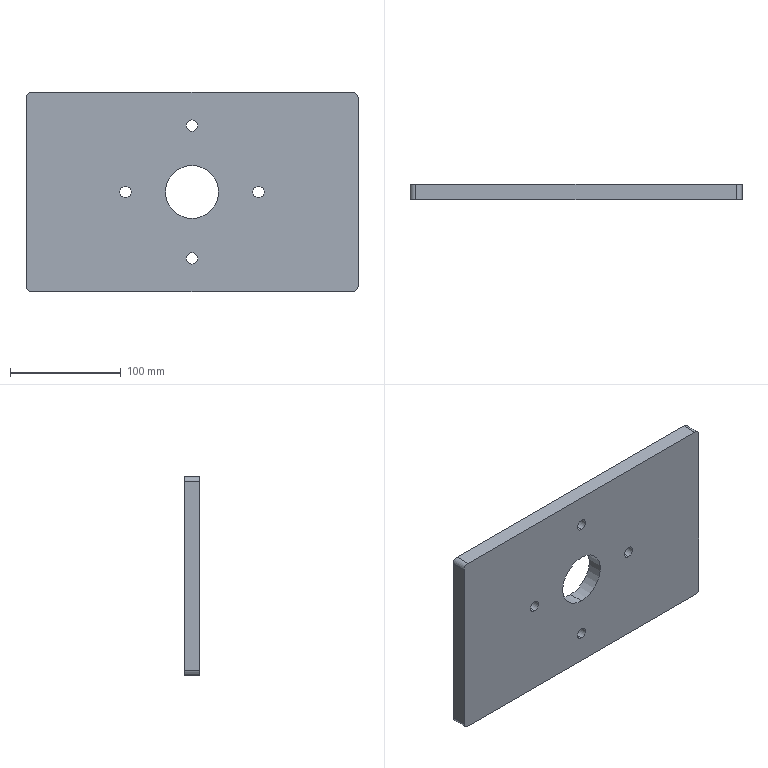Part | SolidWorks | features BaseBody 1 | 1 solid | 20 faces | box 300 x 14 x 180 mm | volume 725790 mm3 | cylinder 14 | plane 6 | commonest cylinder face diameters 10.2 x8 10 x4 48 x2
STEP:
#1=CARTESIAN_POINT('',(0.,0.,-24.));
#2=VERTEX_POINT('',#1);
#3=CARTESIAN_POINT('',(0.,0.,24.));
#4=VERTEX_POINT('',#3);
#5=CARTESIAN_POINT('',(0.,0.,0.));
#6=DIRECTION('',(0.,1.,0.));
#7=DIRECTION('',(0.,0.,1.));
#8=AXIS2_PLACEMENT_3D('',#5,#6,#7);
#9=CIRCLE('',#8,24.);
#10=EDGE_CURVE('',#2,#4,#9,.T.);
#11=ORIENTED_EDGE('',*,*,#10,.F.);
#12=CARTESIAN_POINT('',(0.,14.,-24.));
#13=VERTEX_POINT('',#12);
#14=CARTESIAN_POINT('',(0.,0.,-24.));
#15=DIRECTION('',(0.,1.,0.));
#16=VECTOR('',#15,1000.);
#17=LINE('',#14,#16);
#18=EDGE_CURVE('',#2,#13,#17,.T.);
#19=ORIENTED_EDGE('',*,*,#18,.T.);
#20=CARTESIAN_POINT('',(0.,14.,24.));
#21=VERTEX_POINT('',#20);
#22=CARTESIAN_POINT('',(0.,14.,0.));
#23=DIRECTION('',(0.,1.,0.));
#24=DIRECTION('',(0.,0.,1.));
#25=AXIS2_PLACEMENT_3D('',#22,#23,#24);
#26=CIRCLE('',#25,24.);
#27=EDGE_CURVE('',#13,#21,#26,.T.);
#28=ORIENTED_EDGE('',*,*,#27,.T.);
#29=CARTESIAN_POINT('',(0.,0.,24.));
#30=DIRECTION('',(0.,1.,0.));
#31=VECTOR('',#30,1000.);
#32=LINE('',#29,#31);
#33=EDGE_CURVE('',#4,#21,#32,.T.);
#34=ORIENTED_EDGE('',*,*,#33,.F.);
#35=EDGE_LOOP('',(#11,#19,#28,#34));
#36=FACE_OUTER_BOUND('',#35,.T.);
#37=CARTESIAN_POINT('',(0.,0.,0.));
#38=DIRECTION('',(0.,1.,0.));
#39=DIRECTION('',(0.,0.,1.));
#40=AXIS2_PLACEMENT_3D('',#37,#38,#39);
#41=CYLINDRICAL_SURFACE('',#40,24.);
#42=ADVANCED_FACE('',(#36),#41,.F.);
#43=CARTESIAN_POINT('',(0.,0.,-65.1));
#44=VERTEX_POINT('',#43);
#45=CARTESIAN_POINT('',(0.,0.,-54.9));
#46=VERTEX_POINT('',#45);
#47=CARTESIAN_POINT('',(0.,0.,-60.));
#48=DIRECTION('',(0.,1.,0.));
#49=DIRECTION('',(0.,0.,1.));
#50=AXIS2_PLACEMENT_3D('',#47,#48,#49);
#51=CIRCLE('',#50,5.1);
#52=EDGE_CURVE('',#44,#46,#51,.T.);
#53=ORIENTED_EDGE('',*,*,#52,.F.);
#54=CARTESIAN_POINT('',(0.,14.,-65.1));
#55=VERTEX_POINT('',#54);
#56=CARTESIAN_POINT('',(0.,14.,-65.1));
#57=DIRECTION('',(0.,1.,0.));
#58=VECTOR('',#57,1000.);
#59=LINE('',#56,#58);
#60=EDGE_CURVE('',#44,#55,#59,.T.);
#61=ORIENTED_EDGE('',*,*,#60,.T.);
#62=CARTESIAN_POINT('',(0.,14.,-54.9));
#63=VERTEX_POINT('',#62);
#64=CARTESIAN_POINT('',(0.,14.,-60.));
#65=DIRECTION('',(0.,1.,0.));
#66=DIRECTION('',(0.,0.,1.));
#67=AXIS2_PLACEMENT_3D('',#64,#65,#66);
#68=CIRCLE('',#67,5.1);
#69=EDGE_CURVE('',#55,#63,#68,.T.);
#70=ORIENTED_EDGE('',*,*,#69,.T.);
#71=CARTESIAN_POINT('',(0.,14.,-54.9));
#72=DIRECTION('',(0.,1.,0.));
#73=VECTOR('',#72,1000.);
#74=LINE('',#71,#73);
#75=EDGE_CURVE('',#46,#63,#74,.T.);
#76=ORIENTED_EDGE('',*,*,#75,.F.);
#77=EDGE_LOOP('',(#53,#61,#70,#76));
#78=FACE_OUTER_BOUND('',#77,.T.);
#79=CARTESIAN_POINT('',(0.,14.,-60.));
#80=DIRECTION('',(0.,1.,0.));
#81=DIRECTION('',(0.,0.,1.));
#82=AXIS2_PLACEMENT_3D('',#79,#80,#81);
#83=CYLINDRICAL_SURFACE('',#82,5.1);
#84=ADVANCED_FACE('',(#78),#83,.F.);
#85=CARTESIAN_POINT('',(-60.,0.,-5.1));
#86=VERTEX_POINT('',#85);
#87=CARTESIAN_POINT('',(-60.,0.,5.1));
#88=VERTEX_POINT('',#87);
#89=CARTESIAN_POINT('',(-60.,0.,0.));
#90=DIRECTION('',(0.,1.,0.));
#91=DIRECTION('',(0.,0.,1.));
#92=AXIS2_PLACEMENT_3D('',#89,#90,#91);
#93=CIRCLE('',#92,5.1);
#94=EDGE_CURVE('',#86,#88,#93,.T.);
#95=ORIENTED_EDGE('',*,*,#94,.F.);
#96=CARTESIAN_POINT('',(-60.,14.,-5.1));
#97=VERTEX_POINT('',#96);
#98=CARTESIAN_POINT('',(-60.,14.,-5.1));
#99=DIRECTION('',(0.,1.,0.));
#100=VECTOR('',#99,1000.);
#101=LINE('',#98,#100);
#102=EDGE_CURVE('',#86,#97,#101,.T.);
#103=ORIENTED_EDGE('',*,*,#102,.T.);
#104=CARTESIAN_POINT('',(-60.,14.,5.1));
#105=VERTEX_POINT('',#104);
#106=CARTESIAN_POINT('',(-60.,14.,0.));
#107=DIRECTION('',(0.,1.,0.));
#108=DIRECTION('',(0.,0.,1.));
#109=AXIS2_PLACEMENT_3D('',#106,#107,#108);
#110=CIRCLE('',#109,5.1);
#111=EDGE_CURVE('',#97,#105,#110,.T.);
#112=ORIENTED_EDGE('',*,*,#111,.T.);
#113=CARTESIAN_POINT('',(-60.,14.,5.1));
#114=DIRECTION('',(0.,1.,0.));
#115=VECTOR('',#114,1000.);
#116=LINE('',#113,#115);
#117=EDGE_CURVE('',#88,#105,#116,.T.);
#118=ORIENTED_EDGE('',*,*,#117,.F.);
#119=EDGE_LOOP('',(#95,#103,#112,#118));
#120=FACE_OUTER_BOUND('',#119,.T.);
#121=CARTESIAN_POINT('',(-60.,14.,0.));
#122=DIRECTION('',(0.,1.,0.));
#123=DIRECTION('',(0.,0.,1.));
#124=AXIS2_PLACEMENT_3D('',#121,#122,#123);
#125=CYLINDRICAL_SURFACE('',#124,5.1);
#126=ADVANCED_FACE('',(#120),#125,.F.);
#127=CARTESIAN_POINT('',(0.,0.,54.9));
#128=VERTEX_POINT('',#127);
#129=CARTESIAN_POINT('',(0.,0.,65.1));
#130=VERTEX_POINT('',#129);
#131=CARTESIAN_POINT('',(0.,0.,60.));
#132=DIRECTION('',(0.,1.,0.));
#133=DIRECTION('',(0.,0.,1.));
#134=AXIS2_PLACEMENT_3D('',#131,#132,#133);
#135=CIRCLE('',#134,5.1);
#136=EDGE_CURVE('',#128,#130,#135,.T.);
#137=ORIENTED_EDGE('',*,*,#136,.F.);
#138=CARTESIAN_POINT('',(0.,14.,54.9));
#139=VERTEX_POINT('',#138);
#140=CARTESIAN_POINT('',(0.,14.,54.9));
#141=DIRECTION('',(0.,1.,0.));
#142=VECTOR('',#141,1000.);
#143=LINE('',#140,#142);
#144=EDGE_CURVE('',#128,#139,#143,.T.);
#145=ORIENTED_EDGE('',*,*,#144,.T.);
#146=CARTESIAN_POINT('',(0.,14.,65.1));
#147=VERTEX_POINT('',#146);
#148=CARTESIAN_POINT('',(0.,14.,60.));
#149=DIRECTION('',(0.,1.,0.));
#150=DIRECTION('',(0.,0.,1.));
#151=AXIS2_PLACEMENT_3D('',#148,#149,#150);
#152=CIRCLE('',#151,5.1);
#153=EDGE_CURVE('',#139,#147,#152,.T.);
#154=ORIENTED_EDGE('',*,*,#153,.T.);
#155=CARTESIAN_POINT('',(0.,14.,65.1));
#156=DIRECTION('',(0.,1.,0.));
#157=VECTOR('',#156,1000.);
#158=LINE('',#155,#157);
#159=EDGE_CURVE('',#130,#147,#158,.T.);
#160=ORIENTED_EDGE('',*,*,#159,.F.);
#161=EDGE_LOOP('',(#137,#145,#154,#160));
#162=FACE_OUTER_BOUND('',#161,.T.);
#163=CARTESIAN_POINT('',(0.,14.,60.));
#164=DIRECTION('',(0.,1.,0.));
#165=DIRECTION('',(0.,0.,1.));
#166=AXIS2_PLACEMENT_3D('',#163,#164,#165);
#167=CYLINDRICAL_SURFACE('',#166,5.1);
#168=ADVANCED_FACE('',(#162),#167,.F.);
#169=CARTESIAN_POINT('',(60.,0.,-5.1));
#170=VERTEX_POINT('',#169);
#171=CARTESIAN_POINT('',(60.,0.,5.1));
#172=VERTEX_POINT('',#171);
#173=CARTESIAN_POINT('',(60.,0.,0.));
#174=DIRECTION('',(0.,1.,0.));
#175=DIRECTION('',(0.,0.,1.));
#176=AXIS2_PLACEMENT_3D('',#173,#174,#175);
#177=CIRCLE('',#176,5.1);
#178=EDGE_CURVE('',#170,#172,#177,.T.);
#179=ORIENTED_EDGE('',*,*,#178,.F.);
#180=CARTESIAN_POINT('',(60.,14.,-5.1));
#181=VERTEX_POINT('',#180);
#182=CARTESIAN_POINT('',(60.,14.,-5.1));
#183=DIRECTION('',(0.,1.,0.));
#184=VECTOR('',#183,1000.);
#185=LINE('',#182,#184);
#186=EDGE_CURVE('',#170,#181,#185,.T.);
#187=ORIENTED_EDGE('',*,*,#186,.T.);
#188=CARTESIAN_POINT('',(60.,14.,5.1));
#189=VERTEX_POINT('',#188);
#190=CARTESIAN_POINT('',(60.,14.,0.));
#191=DIRECTION('',(0.,1.,0.));
#192=DIRECTION('',(0.,0.,1.));
#193=AXIS2_PLACEMENT_3D('',#190,#191,#192);
#194=CIRCLE('',#193,5.1);
#195=EDGE_CURVE('',#181,#189,#194,.T.);
#196=ORIENTED_EDGE('',*,*,#195,.T.);
#197=CARTESIAN_POINT('',(60.,14.,5.1));
#198=DIRECTION('',(0.,1.,0.));
#199=VECTOR('',#198,1000.);
#200=LINE('',#197,#199);
#201=EDGE_CURVE('',#172,#189,#200,.T.);
#202=ORIENTED_EDGE('',*,*,#201,.F.);
#203=EDGE_LOOP('',(#179,#187,#196,#202));
#204=FACE_OUTER_BOUND('',#203,.T.);
#205=CARTESIAN_POINT('',(60.,14.,0.));
#206=DIRECTION('',(0.,1.,0.));
#207=DIRECTION('',(0.,0.,1.));
#208=AXIS2_PLACEMENT_3D('',#205,#206,#207);
#209=CYLINDRICAL_SURFACE('',#208,5.1);
#210=ADVANCED_FACE('',(#204),#209,.F.);
#211=CARTESIAN_POINT('',(145.,14.,-90.));
#212=VERTEX_POINT('',#211);
#213=CARTESIAN_POINT('',(150.,14.,-85.));
#214=VERTEX_POINT('',#213);
#215=CARTESIAN_POINT('',(145.,14.,-85.));
#216=DIRECTION('',(0.,-1.,0.));
#217=DIRECTION('',(0.,0.,-1.));
#218=AXIS2_PLACEMENT_3D('',#215,#216,#217);
#219=CIRCLE('',#218,5.);
#220=EDGE_CURVE('',#212,#214,#219,.T.);
#221=ORIENTED_EDGE('',*,*,#220,.F.);
#222=CARTESIAN_POINT('',(-145.,14.,-90.));
#223=VERTEX_POINT('',#222);
#224=CARTESIAN_POINT('',(0.,14.,-90.));
#225=DIRECTION('',(1.,0.,0.));
#226=VECTOR('',#225,1000.);
#227=LINE('',#224,#226);
#228=EDGE_CURVE('',#223,#212,#227,.T.);
#229=ORIENTED_EDGE('',*,*,#228,.F.);
#230=CARTESIAN_POINT('',(-150.,14.,-85.));
#231=VERTEX_POINT('',#230);
#232=CARTESIAN_POINT('',(-145.,14.,-85.));
#233=DIRECTION('',(0.,-1.,0.));
#234=DIRECTION('',(0.,0.,-1.));
#235=AXIS2_PLACEMENT_3D('',#232,#233,#234);
#236=CIRCLE('',#235,5.);
#237=EDGE_CURVE('',#231,#223,#236,.T.);
#238=ORIENTED_EDGE('',*,*,#237,.F.);
#239=CARTESIAN_POINT('',(-150.,14.,85.));
#240=VERTEX_POINT('',#239);
#241=CARTESIAN_POINT('',(-150.,14.,0.));
#242=DIRECTION('',(0.,0.,-1.));
#243=VECTOR('',#242,1000.);
#244=LINE('',#241,#243);
#245=EDGE_CURVE('',#240,#231,#244,.T.);
#246=ORIENTED_EDGE('',*,*,#245,.F.);
#247=CARTESIAN_POINT('',(-145.,14.,90.));
#248=VERTEX_POINT('',#247);
#249=CARTESIAN_POINT('',(-145.,14.,85.));
#250=DIRECTION('',(0.,-1.,0.));
#251=DIRECTION('',(0.,0.,-1.));
#252=AXIS2_PLACEMENT_3D('',#249,#250,#251);
#253=CIRCLE('',#252,5.);
#254=EDGE_CURVE('',#248,#240,#253,.T.);
#255=ORIENTED_EDGE('',*,*,#254,.F.);
#256=CARTESIAN_POINT('',(145.,14.,90.));
#257=VERTEX_POINT('',#256);
#258=CARTESIAN_POINT('',(0.,14.,90.));
#259=DIRECTION('',(-1.,0.,0.));
#260=VECTOR('',#259,1000.);
#261=LINE('',#258,#260);
#262=EDGE_CURVE('',#257,#248,#261,.T.);
#263=ORIENTED_EDGE('',*,*,#262,.F.);
#264=CARTESIAN_POINT('',(150.,14.,85.));
#265=VERTEX_POINT('',#264);
#266=CARTESIAN_POINT('',(145.,14.,85.));
#267=DIRECTION('',(0.,-1.,0.));
#268=DIRECTION('',(0.,0.,-1.));
#269=AXIS2_PLACEMENT_3D('',#266,#267,#268);
#270=CIRCLE('',#269,5.);
#271=EDGE_CURVE('',#265,#257,#270,.T.);
#272=ORIENTED_EDGE('',*,*,#271,.F.);
#273=CARTESIAN_POINT('',(150.,14.,0.));
#274=DIRECTION('',(0.,0.,1.));
#275=VECTOR('',#274,1000.);
#276=LINE('',#273,#275);
#277=EDGE_CURVE('',#214,#265,#276,.T.);
#278=ORIENTED_EDGE('',*,*,#277,.F.);
#279=EDGE_LOOP('',(#221,#229,#238,#246,#255,#263,#272,#278));
#280=FACE_OUTER_BOUND('',#279,.T.);
#281=CARTESIAN_POINT('',(0.,14.,0.));
#282=DIRECTION('',(0.,1.,0.));
#283=DIRECTION('',(0.,0.,1.));
#284=AXIS2_PLACEMENT_3D('',#281,#282,#283);
#285=CIRCLE('',#284,24.);
#286=EDGE_CURVE('',#21,#13,#285,.T.);
#287=ORIENTED_EDGE('',*,*,#286,.F.);
#288=ORIENTED_EDGE('',*,*,#27,.F.);
#289=EDGE_LOOP('',(#287,#288));
#290=FACE_BOUND('',#289,.T.);
#291=CARTESIAN_POINT('',(0.,14.,-60.));
#292=DIRECTION('',(0.,1.,0.));
#293=DIRECTION('',(0.,0.,1.));
#294=AXIS2_PLACEMENT_3D('',#291,#292,#293);
#295=CIRCLE('',#294,5.1);
#296=EDGE_CURVE('',#63,#55,#295,.T.);
#297=ORIENTED_EDGE('',*,*,#296,.F.);
#298=ORIENTED_EDGE('',*,*,#69,.F.);
#299=EDGE_LOOP('',(#297,#298));
#300=FACE_BOUND('',#299,.T.);
#301=CARTESIAN_POINT('',(-60.,14.,0.));
#302=DIRECTION('',(0.,1.,0.));
#303=DIRECTION('',(0.,0.,1.));
#304=AXIS2_PLACEMENT_3D('',#301,#302,#303);
#305=CIRCLE('',#304,5.1);
#306=EDGE_CURVE('',#105,#97,#305,.T.);
#307=ORIENTED_EDGE('',*,*,#306,.F.);
#308=ORIENTED_EDGE('',*,*,#111,.F.);
#309=EDGE_LOOP('',(#307,#308));
#310=FACE_BOUND('',#309,.T.);
#311=CARTESIAN_POINT('',(0.,14.,60.));
#312=DIRECTION('',(0.,1.,0.));
#313=DIRECTION('',(0.,0.,1.));
#314=AXIS2_PLACEMENT_3D('',#311,#312,#313);
#315=CIRCLE('',#314,5.1);
#316=EDGE_CURVE('',#147,#139,#315,.T.);
#317=ORIENTED_EDGE('',*,*,#316,.F.);
#318=ORIENTED_EDGE('',*,*,#153,.F.);
#319=EDGE_LOOP('',(#317,#318));
#320=FACE_BOUND('',#319,.T.);
#321=CARTESIAN_POINT('',(60.,14.,0.));
#322=DIRECTION('',(0.,1.,0.));
#323=DIRECTION('',(0.,0.,1.));
#324=AXIS2_PLACEMENT_3D('',#321,#322,#323);
#325=CIRCLE('',#324,5.1);
#326=EDGE_CURVE('',#189,#181,#325,.T.);
#327=ORIENTED_EDGE('',*,*,#326,.F.);
#328=ORIENTED_EDGE('',*,*,#195,.F.);
#329=EDGE_LOOP('',(#327,#328));
#330=FACE_BOUND('',#329,.T.);
#331=CARTESIAN_POINT('',(0.,14.,0.));
#332=DIRECTION('',(0.,-1.,0.));
#333=DIRECTION('',(0.,0.,-1.));
#334=AXIS2_PLACEMENT_3D('',#331,#332,#333);
#335=PLANE('',#334);
#336=ADVANCED_FACE('',(#280,#290,#300,#310,#320,#330),#335,.F.);
#337=CARTESIAN_POINT('',(150.,0.,-85.));
#338=VERTEX_POINT('',#337);
#339=CARTESIAN_POINT('',(150.,14.,-85.));
#340=DIRECTION('',(0.,-1.,0.));
#341=VECTOR('',#340,1000.);
#342=LINE('',#339,#341);
#343=EDGE_CURVE('',#214,#338,#342,.T.);
#344=ORIENTED_EDGE('',*,*,#343,.F.);
#345=ORIENTED_EDGE('',*,*,#277,.T.);
#346=CARTESIAN_POINT('',(150.,0.,85.));
#347=VERTEX_POINT('',#346);
#348=CARTESIAN_POINT('',(150.,14.,85.));
#349=DIRECTION('',(0.,1.,0.));
#350=VECTOR('',#349,1000.);
#351=LINE('',#348,#350);
#352=EDGE_CURVE('',#347,#265,#351,.T.);
#353=ORIENTED_EDGE('',*,*,#352,.F.);
#354=CARTESIAN_POINT('',(150.,0.,90.));
#355=DIRECTION('',(0.,0.,1.));
#356=VECTOR('',#355,1000.);
#357=LINE('',#354,#356);
#358=EDGE_CURVE('',#338,#347,#357,.T.);
#359=ORIENTED_EDGE('',*,*,#358,.F.);
#360=EDGE_LOOP('',(#344,#345,#353,#359));
#361=FACE_OUTER_BOUND('',#360,.T.);
#362=CARTESIAN_POINT('',(150.,14.,90.));
#363=DIRECTION('',(-1.,0.,0.));
#364=DIRECTION('',(0.,0.,1.));
#365=AXIS2_PLACEMENT_3D('',#362,#363,#364);
#366=PLANE('',#365);
#367=ADVANCED_FACE('',(#361),#366,.F.);
#368=CARTESIAN_POINT('',(145.,0.,-90.));
#369=VERTEX_POINT('',#368);
#370=CARTESIAN_POINT('',(145.,0.,-85.));
#371=DIRECTION('',(0.,1.,0.));
#372=DIRECTION('',(0.,0.,-1.));
#373=AXIS2_PLACEMENT_3D('',#370,#371,#372);
#374=CIRCLE('',#373,5.);
#375=EDGE_CURVE('',#338,#369,#374,.T.);
#376=ORIENTED_EDGE('',*,*,#375,.T.);
#377=CARTESIAN_POINT('',(145.,14.,-90.));
#378=DIRECTION('',(0.,1.,0.));
#379=VECTOR('',#378,1000.);
#380=LINE('',#377,#379);
#381=EDGE_CURVE('',#369,#212,#380,.T.);
#382=ORIENTED_EDGE('',*,*,#381,.T.);
#383=ORIENTED_EDGE('',*,*,#220,.T.);
#384=ORIENTED_EDGE('',*,*,#343,.T.);
#385=EDGE_LOOP('',(#376,#382,#383,#384));
#386=FACE_OUTER_BOUND('',#385,.T.);
#387=CARTESIAN_POINT('',(145.,14.,-85.));
#388=DIRECTION('',(0.,-1.,0.));
#389=DIRECTION('',(0.,0.,-1.));
#390=AXIS2_PLACEMENT_3D('',#387,#388,#389);
#391=CYLINDRICAL_SURFACE('',#390,5.);
#392=ADVANCED_FACE('',(#386),#391,.T.);
#393=ORIENTED_EDGE('',*,*,#381,.F.);
#394=CARTESIAN_POINT('',(-145.,0.,-90.));
#395=VERTEX_POINT('',#394);
#396=CARTESIAN_POINT('',(-150.,0.,-90.));
#397=DIRECTION('',(1.,0.,0.));
#398=VECTOR('',#397,1000.);
#399=LINE('',#396,#398);
#400=EDGE_CURVE('',#395,#369,#399,.T.);
#401=ORIENTED_EDGE('',*,*,#400,.F.);
#402=CARTESIAN_POINT('',(-145.,14.,-90.));
#403=DIRECTION('',(0.,-1.,0.));
#404=VECTOR('',#403,1000.);
#405=LINE('',#402,#404);
#406=EDGE_CURVE('',#223,#395,#405,.T.);
#407=ORIENTED_EDGE('',*,*,#406,.F.);
#408=ORIENTED_EDGE('',*,*,#228,.T.);
#409=EDGE_LOOP('',(#393,#401,#407,#408));
#410=FACE_OUTER_BOUND('',#409,.T.);
#411=CARTESIAN_POINT('',(-150.,14.,-90.));
#412=DIRECTION('',(0.,0.,1.));
#413=DIRECTION('',(1.,0.,0.));
#414=AXIS2_PLACEMENT_3D('',#411,#412,#413);
#415=PLANE('',#414);
#416=ADVANCED_FACE('',(#410),#415,.F.);
#417=CARTESIAN_POINT('',(-150.,0.,-85.));
#418=VERTEX_POINT('',#417);
#419=CARTESIAN_POINT('',(-145.,0.,-85.));
#420=DIRECTION('',(0.,1.,0.));
#421=DIRECTION('',(0.,0.,-1.));
#422=AXIS2_PLACEMENT_3D('',#419,#420,#421);
#423=CIRCLE('',#422,5.);
#424=EDGE_CURVE('',#395,#418,#423,.T.);
#425=ORIENTED_EDGE('',*,*,#424,.T.);
#426=CARTESIAN_POINT('',(-150.,14.,-85.));
#427=DIRECTION('',(0.,1.,0.));
#428=VECTOR('',#427,1000.);
#429=LINE('',#426,#428);
#430=EDGE_CURVE('',#418,#231,#429,.T.);
#431=ORIENTED_EDGE('',*,*,#430,.T.);
#432=ORIENTED_EDGE('',*,*,#237,.T.);
#433=ORIENTED_EDGE('',*,*,#406,.T.);
#434=EDGE_LOOP('',(#425,#431,#432,#433));
#435=FACE_OUTER_BOUND('',#434,.T.);
#436=CARTESIAN_POINT('',(-145.,14.,-85.));
#437=DIRECTION('',(0.,-1.,0.));
#438=DIRECTION('',(0.,0.,-1.));
#439=AXIS2_PLACEMENT_3D('',#436,#437,#438);
#440=CYLINDRICAL_SURFACE('',#439,5.);
#441=ADVANCED_FACE('',(#435),#440,.T.);
#442=CARTESIAN_POINT('',(-150.,0.,85.));
#443=VERTEX_POINT('',#442);
#444=CARTESIAN_POINT('',(-150.,14.,85.));
#445=DIRECTION('',(0.,-1.,0.));
#446=VECTOR('',#445,1000.);
#447=LINE('',#444,#446);
#448=EDGE_CURVE('',#240,#443,#447,.T.);
#449=ORIENTED_EDGE('',*,*,#448,.F.);
#450=ORIENTED_EDGE('',*,*,#245,.T.);
#451=ORIENTED_EDGE('',*,*,#430,.F.);
#452=CARTESIAN_POINT('',(-150.,0.,90.));
#453=DIRECTION('',(0.,0.,-1.));
#454=VECTOR('',#453,1000.);
#455=LINE('',#452,#454);
#456=EDGE_CURVE('',#443,#418,#455,.T.);
#457=ORIENTED_EDGE('',*,*,#456,.F.);
#458=EDGE_LOOP('',(#449,#450,#451,#457));
#459=FACE_OUTER_BOUND('',#458,.T.);
#460=CARTESIAN_POINT('',(-150.,14.,90.));
#461=DIRECTION('',(1.,0.,0.));
#462=DIRECTION('',(0.,0.,-1.));
#463=AXIS2_PLACEMENT_3D('',#460,#461,#462);
#464=PLANE('',#463);
#465=ADVANCED_FACE('',(#459),#464,.F.);
#466=CARTESIAN_POINT('',(-145.,0.,90.));
#467=VERTEX_POINT('',#466);
#468=CARTESIAN_POINT('',(-145.,0.,85.));
#469=DIRECTION('',(0.,1.,0.));
#470=DIRECTION('',(0.,0.,-1.));
#471=AXIS2_PLACEMENT_3D('',#468,#469,#470);
#472=CIRCLE('',#471,5.);
#473=EDGE_CURVE('',#443,#467,#472,.T.);
#474=ORIENTED_EDGE('',*,*,#473,.T.);
#475=CARTESIAN_POINT('',(-145.,14.,90.));
#476=DIRECTION('',(0.,1.,0.));
#477=VECTOR('',#476,1000.);
#478=LINE('',#475,#477);
#479=EDGE_CURVE('',#467,#248,#478,.T.);
#480=ORIENTED_EDGE('',*,*,#479,.T.);
#481=ORIENTED_EDGE('',*,*,#254,.T.);
#482=ORIENTED_EDGE('',*,*,#448,.T.);
#483=EDGE_LOOP('',(#474,#480,#481,#482));
#484=FACE_OUTER_BOUND('',#483,.T.);
#485=CARTESIAN_POINT('',(-145.,14.,85.));
#486=DIRECTION('',(0.,-1.,0.));
#487=DIRECTION('',(0.,0.,-1.));
#488=AXIS2_PLACEMENT_3D('',#485,#486,#487);
#489=CYLINDRICAL_SURFACE('',#488,5.);
#490=ADVANCED_FACE('',(#484),#489,.T.);
#491=CARTESIAN_POINT('',(145.,0.,90.));
#492=VERTEX_POINT('',#491);
#493=CARTESIAN_POINT('',(145.,14.,90.));
#494=DIRECTION('',(0.,-1.,0.));
#495=VECTOR('',#494,1000.);
#496=LINE('',#493,#495);
#497=EDGE_CURVE('',#257,#492,#496,.T.);
#498=ORIENTED_EDGE('',*,*,#497,.F.);
#499=ORIENTED_EDGE('',*,*,#262,.T.);
#500=ORIENTED_EDGE('',*,*,#479,.F.);
#501=CARTESIAN_POINT('',(-150.,0.,90.));
#502=DIRECTION('',(-1.,0.,0.));
#503=VECTOR('',#502,1000.);
#504=LINE('',#501,#503);
#505=EDGE_CURVE('',#492,#467,#504,.T.);
#506=ORIENTED_EDGE('',*,*,#505,.F.);
#507=EDGE_LOOP('',(#498,#499,#500,#506));
#508=FACE_OUTER_BOUND('',#507,.T.);
#509=CARTESIAN_POINT('',(-150.,14.,90.));
#510=DIRECTION('',(0.,0.,-1.));
#511=DIRECTION('',(-1.,0.,0.));
#512=AXIS2_PLACEMENT_3D('',#509,#510,#511);
#513=PLANE('',#512);
#514=ADVANCED_FACE('',(#508),#513,.F.);
#515=CARTESIAN_POINT('',(145.,0.,85.));
#516=DIRECTION('',(0.,1.,0.));
#517=DIRECTION('',(0.,0.,-1.));
#518=AXIS2_PLACEMENT_3D('',#515,#516,#517);
#519=CIRCLE('',#518,5.);
#520=EDGE_CURVE('',#492,#347,#519,.T.);
#521=ORIENTED_EDGE('',*,*,#520,.T.);
#522=ORIENTED_EDGE('',*,*,#352,.T.);
#523=ORIENTED_EDGE('',*,*,#271,.T.);
#524=ORIENTED_EDGE('',*,*,#497,.T.);
#525=EDGE_LOOP('',(#521,#522,#523,#524));
#526=FACE_OUTER_BOUND('',#525,.T.);
#527=CARTESIAN_POINT('',(145.,14.,85.));
#528=DIRECTION('',(0.,-1.,0.));
#529=DIRECTION('',(0.,0.,-1.));
#530=AXIS2_PLACEMENT_3D('',#527,#528,#529);
#531=CYLINDRICAL_SURFACE('',#530,5.);
#532=ADVANCED_FACE('',(#526),#531,.T.);
#533=ORIENTED_EDGE('',*,*,#18,.F.);
#534=CARTESIAN_POINT('',(0.,0.,0.));
#535=DIRECTION('',(0.,1.,0.));
#536=DIRECTION('',(0.,0.,1.));
#537=AXIS2_PLACEMENT_3D('',#534,#535,#536);
#538=CIRCLE('',#537,24.);
#539=EDGE_CURVE('',#4,#2,#538,.T.);
#540=ORIENTED_EDGE('',*,*,#539,.F.);
#541=ORIENTED_EDGE('',*,*,#33,.T.);
#542=ORIENTED_EDGE('',*,*,#286,.T.);
#543=EDGE_LOOP('',(#533,#540,#541,#542));
#544=FACE_OUTER_BOUND('',#543,.T.);
#545=CARTESIAN_POINT('',(0.,0.,0.));
#546=DIRECTION('',(0.,1.,0.));
#547=DIRECTION('',(0.,0.,1.));
#548=AXIS2_PLACEMENT_3D('',#545,#546,#547);
#549=CYLINDRICAL_SURFACE('',#548,24.);
#550=ADVANCED_FACE('',(#544),#549,.F.);
#551=ORIENTED_EDGE('',*,*,#60,.F.);
#552=CARTESIAN_POINT('',(0.,0.,-60.));
#553=DIRECTION('',(0.,1.,0.));
#554=DIRECTION('',(0.,0.,1.));
#555=AXIS2_PLACEMENT_3D('',#552,#553,#554);
#556=CIRCLE('',#555,5.1);
#557=EDGE_CURVE('',#46,#44,#556,.T.);
#558=ORIENTED_EDGE('',*,*,#557,.F.);
#559=ORIENTED_EDGE('',*,*,#75,.T.);
#560=ORIENTED_EDGE('',*,*,#296,.T.);
#561=EDGE_LOOP('',(#551,#558,#559,#560));
#562=FACE_OUTER_BOUND('',#561,.T.);
#563=CARTESIAN_POINT('',(0.,14.,-60.));
#564=DIRECTION('',(0.,1.,0.));
#565=DIRECTION('',(0.,0.,1.));
#566=AXIS2_PLACEMENT_3D('',#563,#564,#565);
#567=CYLINDRICAL_SURFACE('',#566,5.1);
#568=ADVANCED_FACE('',(#562),#567,.F.);
#569=ORIENTED_EDGE('',*,*,#102,.F.);
#570=CARTESIAN_POINT('',(-60.,0.,0.));
#571=DIRECTION('',(0.,1.,0.));
#572=DIRECTION('',(0.,0.,1.));
#573=AXIS2_PLACEMENT_3D('',#570,#571,#572);
#574=CIRCLE('',#573,5.1);
#575=EDGE_CURVE('',#88,#86,#574,.T.);
#576=ORIENTED_EDGE('',*,*,#575,.F.);
#577=ORIENTED_EDGE('',*,*,#117,.T.);
#578=ORIENTED_EDGE('',*,*,#306,.T.);
#579=EDGE_LOOP('',(#569,#576,#577,#578));
#580=FACE_OUTER_BOUND('',#579,.T.);
#581=CARTESIAN_POINT('',(-60.,14.,0.));
#582=DIRECTION('',(0.,1.,0.));
#583=DIRECTION('',(0.,0.,1.));
#584=AXIS2_PLACEMENT_3D('',#581,#582,#583);
#585=CYLINDRICAL_SURFACE('',#584,5.1);
#586=ADVANCED_FACE('',(#580),#585,.F.);
#587=ORIENTED_EDGE('',*,*,#144,.F.);
#588=CARTESIAN_POINT('',(0.,0.,60.));
#589=DIRECTION('',(0.,1.,0.));
#590=DIRECTION('',(0.,0.,1.));
#591=AXIS2_PLACEMENT_3D('',#588,#589,#590);
#592=CIRCLE('',#591,5.1);
#593=EDGE_CURVE('',#130,#128,#592,.T.);
#594=ORIENTED_EDGE('',*,*,#593,.F.);
#595=ORIENTED_EDGE('',*,*,#159,.T.);
#596=ORIENTED_EDGE('',*,*,#316,.T.);
#597=EDGE_LOOP('',(#587,#594,#595,#596));
#598=FACE_OUTER_BOUND('',#597,.T.);
#599=CARTESIAN_POINT('',(0.,14.,60.));
#600=DIRECTION('',(0.,1.,0.));
#601=DIRECTION('',(0.,0.,1.));
#602=AXIS2_PLACEMENT_3D('',#599,#600,#601);
#603=CYLINDRICAL_SURFACE('',#602,5.1);
#604=ADVANCED_FACE('',(#598),#603,.F.);
#605=ORIENTED_EDGE('',*,*,#186,.F.);
#606=CARTESIAN_POINT('',(60.,0.,0.));
#607=DIRECTION('',(0.,1.,0.));
#608=DIRECTION('',(0.,0.,1.));
#609=AXIS2_PLACEMENT_3D('',#606,#607,#608);
#610=CIRCLE('',#609,5.1);
#611=EDGE_CURVE('',#172,#170,#610,.T.);
#612=ORIENTED_EDGE('',*,*,#611,.F.);
#613=ORIENTED_EDGE('',*,*,#201,.T.);
#614=ORIENTED_EDGE('',*,*,#326,.T.);
#615=EDGE_LOOP('',(#605,#612,#613,#614));
#616=FACE_OUTER_BOUND('',#615,.T.);
#617=CARTESIAN_POINT('',(60.,14.,0.));
#618=DIRECTION('',(0.,1.,0.));
#619=DIRECTION('',(0.,0.,1.));
#620=AXIS2_PLACEMENT_3D('',#617,#618,#619);
#621=CYLINDRICAL_SURFACE('',#620,5.1);
#622=ADVANCED_FACE('',(#616),#621,.F.);
#623=ORIENTED_EDGE('',*,*,#456,.T.);
#624=ORIENTED_EDGE('',*,*,#424,.F.);
#625=ORIENTED_EDGE('',*,*,#400,.T.);
#626=ORIENTED_EDGE('',*,*,#375,.F.);
#627=ORIENTED_EDGE('',*,*,#358,.T.);
#628=ORIENTED_EDGE('',*,*,#520,.F.);
#629=ORIENTED_EDGE('',*,*,#505,.T.);
#630=ORIENTED_EDGE('',*,*,#473,.F.);
#631=EDGE_LOOP('',(#623,#624,#625,#626,#627,#628,#629,#630));
#632=FACE_OUTER_BOUND('',#631,.T.);
#633=ORIENTED_EDGE('',*,*,#539,.T.);
#634=ORIENTED_EDGE('',*,*,#10,.T.);
#635=EDGE_LOOP('',(#633,#634));
#636=FACE_BOUND('',#635,.T.);
#637=ORIENTED_EDGE('',*,*,#557,.T.);
#638=ORIENTED_EDGE('',*,*,#52,.T.);
#639=EDGE_LOOP('',(#637,#638));
#640=FACE_BOUND('',#639,.T.);
#641=ORIENTED_EDGE('',*,*,#575,.T.);
#642=ORIENTED_EDGE('',*,*,#94,.T.);
#643=EDGE_LOOP('',(#641,#642));
#644=FACE_BOUND('',#643,.T.);
#645=ORIENTED_EDGE('',*,*,#593,.T.);
#646=ORIENTED_EDGE('',*,*,#136,.T.);
#647=EDGE_LOOP('',(#645,#646));
#648=FACE_BOUND('',#647,.T.);
#649=ORIENTED_EDGE('',*,*,#611,.T.);
#650=ORIENTED_EDGE('',*,*,#178,.T.);
#651=EDGE_LOOP('',(#649,#650));
#652=FACE_BOUND('',#651,.T.);
#653=CARTESIAN_POINT('',(0.,0.,0.));
#654=DIRECTION('',(0.,-1.,0.));
#655=DIRECTION('',(0.,0.,-1.));
#656=AXIS2_PLACEMENT_3D('',#653,#654,#655);
#657=PLANE('',#656);
#658=ADVANCED_FACE('',(#632,#636,#640,#644,#648,#652),#657,.T.);
#659=CLOSED_SHELL('',(#42,#84,#126,#168,#210,#336,#367,#392,#416,#441,#465,#490,#514,#532,#550,#568,#586,#604,#622,#658));
#660=MANIFOLD_SOLID_BREP('',#659);
#661=CARTESIAN_POINT('',(0.,0.,0.));
#662=DIRECTION('',(0.,0.,1.));
#663=DIRECTION('',(1.,0.,0.));
#664=AXIS2_PLACEMENT_3D('',#661,#662,#663);
#665=(LENGTH_UNIT()NAMED_UNIT(*)SI_UNIT(.MILLI.,.METRE.));
#666=UNCERTAINTY_MEASURE_WITH_UNIT(LENGTH_MEASURE(0.00001),#665,'','');
#667=(NAMED_UNIT(*)PLANE_ANGLE_UNIT()SI_UNIT($,.RADIAN.));
#668=(NAMED_UNIT(*)SI_UNIT($,.STERADIAN.)SOLID_ANGLE_UNIT());
#669=(GEOMETRIC_REPRESENTATION_CONTEXT(3)GLOBAL_UNCERTAINTY_ASSIGNED_CONTEXT((#666))GLOBAL_UNIT_ASSIGNED_CONTEXT((#665,#667,#668))REPRESENTATION_CONTEXT('',''));
#670=ADVANCED_BREP_SHAPE_REPRESENTATION('',(#660,#664),#669);